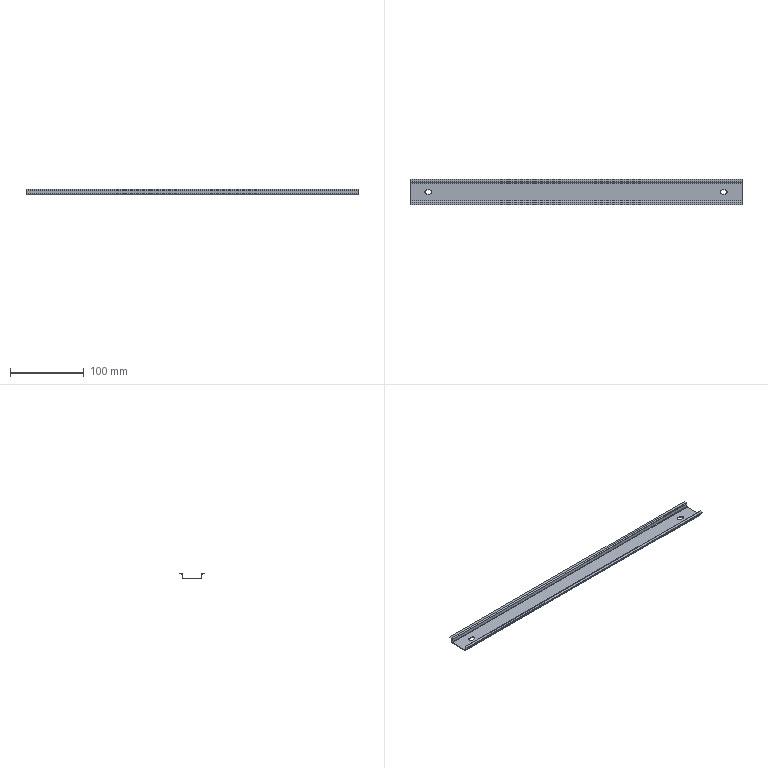Part | SolidWorks | features BaseBody 1 | 1 solid | 48 faces | box 450 x 35 x 7.5 mm | volume 20736 mm3 | plane 34 | cylinder 14 | commonest cylinder face diameters 5.5 x6 1 x4 3 x4
STEP:
#1=CARTESIAN_POINT('',(-202.,-2.75,0.));
#2=VERTEX_POINT('',#1);
#3=CARTESIAN_POINT('',(-198.,-2.75,0.));
#4=VERTEX_POINT('',#3);
#5=CARTESIAN_POINT('',(-202.,-2.75,0.));
#6=DIRECTION('',(1.,0.,0.));
#7=VECTOR('',#6,1000.);
#8=LINE('',#5,#7);
#9=EDGE_CURVE('',#2,#4,#8,.T.);
#10=ORIENTED_EDGE('',*,*,#9,.T.);
#11=CARTESIAN_POINT('',(-198.,-2.75,-1.));
#12=VERTEX_POINT('',#11);
#13=CARTESIAN_POINT('',(-198.,-2.75,-1.));
#14=DIRECTION('',(0.,0.,1.));
#15=VECTOR('',#14,1000.);
#16=LINE('',#13,#15);
#17=EDGE_CURVE('',#12,#4,#16,.T.);
#18=ORIENTED_EDGE('',*,*,#17,.F.);
#19=CARTESIAN_POINT('',(-202.,-2.75,-1.));
#20=VERTEX_POINT('',#19);
#21=CARTESIAN_POINT('',(-202.,-2.75,-1.));
#22=DIRECTION('',(1.,0.,0.));
#23=VECTOR('',#22,1000.);
#24=LINE('',#21,#23);
#25=EDGE_CURVE('',#20,#12,#24,.T.);
#26=ORIENTED_EDGE('',*,*,#25,.F.);
#27=CARTESIAN_POINT('',(-202.,-2.75,-1.));
#28=DIRECTION('',(0.,0.,1.));
#29=VECTOR('',#28,1000.);
#30=LINE('',#27,#29);
#31=EDGE_CURVE('',#20,#2,#30,.T.);
#32=ORIENTED_EDGE('',*,*,#31,.T.);
#33=EDGE_LOOP('',(#10,#18,#26,#32));
#34=FACE_OUTER_BOUND('',#33,.T.);
#35=CARTESIAN_POINT('',(-202.,-2.75,-1.));
#36=DIRECTION('',(0.,-1.,0.));
#37=DIRECTION('',(-1.,0.,0.));
#38=AXIS2_PLACEMENT_3D('',#35,#36,#37);
#39=PLANE('',#38);
#40=ADVANCED_FACE('',(#34),#39,.F.);
#41=CARTESIAN_POINT('',(-195.25,0.,-1.));
#42=VERTEX_POINT('',#41);
#43=CARTESIAN_POINT('',(-195.25,0.,0.));
#44=VERTEX_POINT('',#43);
#45=CARTESIAN_POINT('',(-195.25,0.,-1.));
#46=DIRECTION('',(0.,0.,1.));
#47=VECTOR('',#46,1000.);
#48=LINE('',#45,#47);
#49=EDGE_CURVE('',#42,#44,#48,.T.);
#50=ORIENTED_EDGE('',*,*,#49,.F.);
#51=CARTESIAN_POINT('',(-198.,0.,-1.));
#52=DIRECTION('',(0.,0.,1.));
#53=DIRECTION('',(1.,0.,0.));
#54=AXIS2_PLACEMENT_3D('',#51,#52,#53);
#55=CIRCLE('',#54,2.75);
#56=EDGE_CURVE('',#12,#42,#55,.T.);
#57=ORIENTED_EDGE('',*,*,#56,.F.);
#58=ORIENTED_EDGE('',*,*,#17,.T.);
#59=CARTESIAN_POINT('',(-198.,0.,0.));
#60=DIRECTION('',(0.,0.,1.));
#61=DIRECTION('',(1.,0.,0.));
#62=AXIS2_PLACEMENT_3D('',#59,#60,#61);
#63=CIRCLE('',#62,2.75);
#64=EDGE_CURVE('',#4,#44,#63,.T.);
#65=ORIENTED_EDGE('',*,*,#64,.T.);
#66=EDGE_LOOP('',(#50,#57,#58,#65));
#67=FACE_OUTER_BOUND('',#66,.T.);
#68=CARTESIAN_POINT('',(-198.,0.,-1.));
#69=DIRECTION('',(0.,0.,1.));
#70=DIRECTION('',(1.,0.,0.));
#71=AXIS2_PLACEMENT_3D('',#68,#69,#70);
#72=CYLINDRICAL_SURFACE('',#71,2.75);
#73=ADVANCED_FACE('',(#67),#72,.F.);
#74=CARTESIAN_POINT('',(-198.,2.75,0.));
#75=VERTEX_POINT('',#74);
#76=CARTESIAN_POINT('',(-202.,2.75,0.));
#77=VERTEX_POINT('',#76);
#78=CARTESIAN_POINT('',(-202.,2.75,0.));
#79=DIRECTION('',(-1.,0.,0.));
#80=VECTOR('',#79,1000.);
#81=LINE('',#78,#80);
#82=EDGE_CURVE('',#75,#77,#81,.T.);
#83=ORIENTED_EDGE('',*,*,#82,.T.);
#84=CARTESIAN_POINT('',(-202.,2.75,-1.));
#85=VERTEX_POINT('',#84);
#86=CARTESIAN_POINT('',(-202.,2.75,-1.));
#87=DIRECTION('',(0.,0.,1.));
#88=VECTOR('',#87,1000.);
#89=LINE('',#86,#88);
#90=EDGE_CURVE('',#85,#77,#89,.T.);
#91=ORIENTED_EDGE('',*,*,#90,.F.);
#92=CARTESIAN_POINT('',(-198.,2.75,-1.));
#93=VERTEX_POINT('',#92);
#94=CARTESIAN_POINT('',(-202.,2.75,-1.));
#95=DIRECTION('',(-1.,0.,0.));
#96=VECTOR('',#95,1000.);
#97=LINE('',#94,#96);
#98=EDGE_CURVE('',#93,#85,#97,.T.);
#99=ORIENTED_EDGE('',*,*,#98,.F.);
#100=CARTESIAN_POINT('',(-198.,2.75,-1.));
#101=DIRECTION('',(0.,0.,1.));
#102=VECTOR('',#101,1000.);
#103=LINE('',#100,#102);
#104=EDGE_CURVE('',#93,#75,#103,.T.);
#105=ORIENTED_EDGE('',*,*,#104,.T.);
#106=EDGE_LOOP('',(#83,#91,#99,#105));
#107=FACE_OUTER_BOUND('',#106,.T.);
#108=CARTESIAN_POINT('',(-202.,2.75,-1.));
#109=DIRECTION('',(0.,1.,0.));
#110=DIRECTION('',(1.,0.,0.));
#111=AXIS2_PLACEMENT_3D('',#108,#109,#110);
#112=PLANE('',#111);
#113=ADVANCED_FACE('',(#107),#112,.F.);
#114=CARTESIAN_POINT('',(-202.,0.,0.));
#115=DIRECTION('',(0.,0.,1.));
#116=DIRECTION('',(1.,0.,0.));
#117=AXIS2_PLACEMENT_3D('',#114,#115,#116);
#118=CIRCLE('',#117,2.75);
#119=EDGE_CURVE('',#77,#2,#118,.T.);
#120=ORIENTED_EDGE('',*,*,#119,.T.);
#121=ORIENTED_EDGE('',*,*,#31,.F.);
#122=CARTESIAN_POINT('',(-202.,0.,-1.));
#123=DIRECTION('',(0.,0.,1.));
#124=DIRECTION('',(1.,0.,0.));
#125=AXIS2_PLACEMENT_3D('',#122,#123,#124);
#126=CIRCLE('',#125,2.75);
#127=EDGE_CURVE('',#85,#20,#126,.T.);
#128=ORIENTED_EDGE('',*,*,#127,.F.);
#129=ORIENTED_EDGE('',*,*,#90,.T.);
#130=EDGE_LOOP('',(#120,#121,#128,#129));
#131=FACE_OUTER_BOUND('',#130,.T.);
#132=CARTESIAN_POINT('',(-202.,0.,-1.));
#133=DIRECTION('',(0.,0.,1.));
#134=DIRECTION('',(1.,0.,0.));
#135=AXIS2_PLACEMENT_3D('',#132,#133,#134);
#136=CYLINDRICAL_SURFACE('',#135,2.75);
#137=ADVANCED_FACE('',(#131),#136,.F.);
#138=CARTESIAN_POINT('',(202.,2.75,0.));
#139=VERTEX_POINT('',#138);
#140=CARTESIAN_POINT('',(198.,2.75,0.));
#141=VERTEX_POINT('',#140);
#142=CARTESIAN_POINT('',(202.,2.75,0.));
#143=DIRECTION('',(-1.,0.,0.));
#144=VECTOR('',#143,1000.);
#145=LINE('',#142,#144);
#146=EDGE_CURVE('',#139,#141,#145,.T.);
#147=ORIENTED_EDGE('',*,*,#146,.T.);
#148=CARTESIAN_POINT('',(198.,2.75,-1.));
#149=VERTEX_POINT('',#148);
#150=CARTESIAN_POINT('',(198.,2.75,-1.));
#151=DIRECTION('',(0.,0.,1.));
#152=VECTOR('',#151,1000.);
#153=LINE('',#150,#152);
#154=EDGE_CURVE('',#149,#141,#153,.T.);
#155=ORIENTED_EDGE('',*,*,#154,.F.);
#156=CARTESIAN_POINT('',(202.,2.75,-1.));
#157=VERTEX_POINT('',#156);
#158=CARTESIAN_POINT('',(202.,2.75,-1.));
#159=DIRECTION('',(-1.,0.,0.));
#160=VECTOR('',#159,1000.);
#161=LINE('',#158,#160);
#162=EDGE_CURVE('',#157,#149,#161,.T.);
#163=ORIENTED_EDGE('',*,*,#162,.F.);
#164=CARTESIAN_POINT('',(202.,2.75,-1.));
#165=DIRECTION('',(0.,0.,1.));
#166=VECTOR('',#165,1000.);
#167=LINE('',#164,#166);
#168=EDGE_CURVE('',#157,#139,#167,.T.);
#169=ORIENTED_EDGE('',*,*,#168,.T.);
#170=EDGE_LOOP('',(#147,#155,#163,#169));
#171=FACE_OUTER_BOUND('',#170,.T.);
#172=CARTESIAN_POINT('',(202.,2.75,-1.));
#173=DIRECTION('',(0.,1.,0.));
#174=DIRECTION('',(1.,0.,0.));
#175=AXIS2_PLACEMENT_3D('',#172,#173,#174);
#176=PLANE('',#175);
#177=ADVANCED_FACE('',(#171),#176,.F.);
#178=CARTESIAN_POINT('',(198.,-2.75,0.));
#179=VERTEX_POINT('',#178);
#180=CARTESIAN_POINT('',(198.,0.,0.));
#181=DIRECTION('',(0.,0.,1.));
#182=DIRECTION('',(-1.,0.,0.));
#183=AXIS2_PLACEMENT_3D('',#180,#181,#182);
#184=CIRCLE('',#183,2.75);
#185=EDGE_CURVE('',#141,#179,#184,.T.);
#186=ORIENTED_EDGE('',*,*,#185,.T.);
#187=CARTESIAN_POINT('',(198.,-2.75,-1.));
#188=VERTEX_POINT('',#187);
#189=CARTESIAN_POINT('',(198.,-2.75,-1.));
#190=DIRECTION('',(0.,0.,1.));
#191=VECTOR('',#190,1000.);
#192=LINE('',#189,#191);
#193=EDGE_CURVE('',#188,#179,#192,.T.);
#194=ORIENTED_EDGE('',*,*,#193,.F.);
#195=CARTESIAN_POINT('',(198.,0.,-1.));
#196=DIRECTION('',(0.,0.,1.));
#197=DIRECTION('',(-1.,0.,0.));
#198=AXIS2_PLACEMENT_3D('',#195,#196,#197);
#199=CIRCLE('',#198,2.75);
#200=EDGE_CURVE('',#149,#188,#199,.T.);
#201=ORIENTED_EDGE('',*,*,#200,.F.);
#202=ORIENTED_EDGE('',*,*,#154,.T.);
#203=EDGE_LOOP('',(#186,#194,#201,#202));
#204=FACE_OUTER_BOUND('',#203,.T.);
#205=CARTESIAN_POINT('',(198.,0.,-1.));
#206=DIRECTION('',(0.,0.,1.));
#207=DIRECTION('',(1.,0.,0.));
#208=AXIS2_PLACEMENT_3D('',#205,#206,#207);
#209=CYLINDRICAL_SURFACE('',#208,2.75);
#210=ADVANCED_FACE('',(#204),#209,.F.);
#211=CARTESIAN_POINT('',(202.,-2.75,0.));
#212=VERTEX_POINT('',#211);
#213=CARTESIAN_POINT('',(202.,-2.75,0.));
#214=DIRECTION('',(1.,0.,0.));
#215=VECTOR('',#214,1000.);
#216=LINE('',#213,#215);
#217=EDGE_CURVE('',#179,#212,#216,.T.);
#218=ORIENTED_EDGE('',*,*,#217,.T.);
#219=CARTESIAN_POINT('',(202.,-2.75,-1.));
#220=VERTEX_POINT('',#219);
#221=CARTESIAN_POINT('',(202.,-2.75,-1.));
#222=DIRECTION('',(0.,0.,1.));
#223=VECTOR('',#222,1000.);
#224=LINE('',#221,#223);
#225=EDGE_CURVE('',#220,#212,#224,.T.);
#226=ORIENTED_EDGE('',*,*,#225,.F.);
#227=CARTESIAN_POINT('',(202.,-2.75,-1.));
#228=DIRECTION('',(1.,0.,0.));
#229=VECTOR('',#228,1000.);
#230=LINE('',#227,#229);
#231=EDGE_CURVE('',#188,#220,#230,.T.);
#232=ORIENTED_EDGE('',*,*,#231,.F.);
#233=ORIENTED_EDGE('',*,*,#193,.T.);
#234=EDGE_LOOP('',(#218,#226,#232,#233));
#235=FACE_OUTER_BOUND('',#234,.T.);
#236=CARTESIAN_POINT('',(202.,-2.75,-1.));
#237=DIRECTION('',(0.,-1.,0.));
#238=DIRECTION('',(0.,0.,-1.));
#239=AXIS2_PLACEMENT_3D('',#236,#237,#238);
#240=PLANE('',#239);
#241=ADVANCED_FACE('',(#235),#240,.F.);
#242=CARTESIAN_POINT('',(204.75,0.,-1.));
#243=VERTEX_POINT('',#242);
#244=CARTESIAN_POINT('',(204.75,0.,0.));
#245=VERTEX_POINT('',#244);
#246=CARTESIAN_POINT('',(204.75,0.,-1.));
#247=DIRECTION('',(0.,0.,1.));
#248=VECTOR('',#247,1000.);
#249=LINE('',#246,#248);
#250=EDGE_CURVE('',#243,#245,#249,.T.);
#251=ORIENTED_EDGE('',*,*,#250,.F.);
#252=CARTESIAN_POINT('',(202.,0.,-1.));
#253=DIRECTION('',(0.,0.,1.));
#254=DIRECTION('',(-1.,0.,0.));
#255=AXIS2_PLACEMENT_3D('',#252,#253,#254);
#256=CIRCLE('',#255,2.75);
#257=EDGE_CURVE('',#220,#243,#256,.T.);
#258=ORIENTED_EDGE('',*,*,#257,.F.);
#259=ORIENTED_EDGE('',*,*,#225,.T.);
#260=CARTESIAN_POINT('',(202.,0.,0.));
#261=DIRECTION('',(0.,0.,1.));
#262=DIRECTION('',(-1.,0.,0.));
#263=AXIS2_PLACEMENT_3D('',#260,#261,#262);
#264=CIRCLE('',#263,2.75);
#265=EDGE_CURVE('',#212,#245,#264,.T.);
#266=ORIENTED_EDGE('',*,*,#265,.T.);
#267=EDGE_LOOP('',(#251,#258,#259,#266));
#268=FACE_OUTER_BOUND('',#267,.T.);
#269=CARTESIAN_POINT('',(202.,0.,-1.));
#270=DIRECTION('',(0.,0.,1.));
#271=DIRECTION('',(1.,0.,0.));
#272=AXIS2_PLACEMENT_3D('',#269,#270,#271);
#273=CYLINDRICAL_SURFACE('',#272,2.75);
#274=ADVANCED_FACE('',(#268),#273,.F.);
#275=CARTESIAN_POINT('',(-225.,-17.5,5.5));
#276=VERTEX_POINT('',#275);
#277=CARTESIAN_POINT('',(225.,-17.5,5.5));
#278=VERTEX_POINT('',#277);
#279=CARTESIAN_POINT('',(225.,-17.5,5.5));
#280=DIRECTION('',(1.,0.,0.));
#281=VECTOR('',#280,1000.);
#282=LINE('',#279,#281);
#283=EDGE_CURVE('',#276,#278,#282,.T.);
#284=ORIENTED_EDGE('',*,*,#283,.T.);
#285=CARTESIAN_POINT('',(225.,-17.5,6.5));
#286=VERTEX_POINT('',#285);
#287=CARTESIAN_POINT('',(225.,-17.5,6.5));
#288=DIRECTION('',(0.,0.,-1.));
#289=VECTOR('',#288,1000.);
#290=LINE('',#287,#289);
#291=EDGE_CURVE('',#286,#278,#290,.T.);
#292=ORIENTED_EDGE('',*,*,#291,.F.);
#293=CARTESIAN_POINT('',(-225.,-17.5,6.5));
#294=VERTEX_POINT('',#293);
#295=CARTESIAN_POINT('',(0.,-17.5,6.5));
#296=DIRECTION('',(1.,0.,0.));
#297=VECTOR('',#296,1000.);
#298=LINE('',#295,#297);
#299=EDGE_CURVE('',#294,#286,#298,.T.);
#300=ORIENTED_EDGE('',*,*,#299,.F.);
#301=CARTESIAN_POINT('',(-225.,-17.5,6.5));
#302=DIRECTION('',(0.,0.,-1.));
#303=VECTOR('',#302,1000.);
#304=LINE('',#301,#303);
#305=EDGE_CURVE('',#294,#276,#304,.T.);
#306=ORIENTED_EDGE('',*,*,#305,.T.);
#307=EDGE_LOOP('',(#284,#292,#300,#306));
#308=FACE_OUTER_BOUND('',#307,.T.);
#309=CARTESIAN_POINT('',(225.,-17.5,6.5));
#310=DIRECTION('',(0.,1.,0.));
#311=DIRECTION('',(1.,0.,0.));
#312=AXIS2_PLACEMENT_3D('',#309,#310,#311);
#313=PLANE('',#312);
#314=ADVANCED_FACE('',(#308),#313,.F.);
#315=CARTESIAN_POINT('',(-225.,-14.,5.5));
#316=VERTEX_POINT('',#315);
#317=CARTESIAN_POINT('',(-225.,-17.5,5.5));
#318=DIRECTION('',(0.,-1.,0.));
#319=VECTOR('',#318,1000.);
#320=LINE('',#317,#319);
#321=EDGE_CURVE('',#316,#276,#320,.T.);
#322=ORIENTED_EDGE('',*,*,#321,.F.);
#323=CARTESIAN_POINT('',(225.,-14.,5.5));
#324=VERTEX_POINT('',#323);
#325=CARTESIAN_POINT('',(225.,-14.,5.5));
#326=DIRECTION('',(-1.,0.,0.));
#327=VECTOR('',#326,1000.);
#328=LINE('',#325,#327);
#329=EDGE_CURVE('',#324,#316,#328,.T.);
#330=ORIENTED_EDGE('',*,*,#329,.F.);
#331=CARTESIAN_POINT('',(225.,-13.5,5.5));
#332=DIRECTION('',(0.,1.,0.));
#333=VECTOR('',#332,1000.);
#334=LINE('',#331,#333);
#335=EDGE_CURVE('',#278,#324,#334,.T.);
#336=ORIENTED_EDGE('',*,*,#335,.F.);
#337=ORIENTED_EDGE('',*,*,#283,.F.);
#338=EDGE_LOOP('',(#322,#330,#336,#337));
#339=FACE_OUTER_BOUND('',#338,.T.);
#340=CARTESIAN_POINT('',(0.,0.,5.5));
#341=DIRECTION('',(0.,0.,-1.));
#342=DIRECTION('',(0.,-1.,0.));
#343=AXIS2_PLACEMENT_3D('',#340,#341,#342);
#344=PLANE('',#343);
#345=ADVANCED_FACE('',(#339),#344,.T.);
#346=CARTESIAN_POINT('',(-225.,-14.,6.5));
#347=VERTEX_POINT('',#346);
#348=CARTESIAN_POINT('',(225.,-14.,6.5));
#349=VERTEX_POINT('',#348);
#350=CARTESIAN_POINT('',(225.,-14.,6.5));
#351=DIRECTION('',(1.,0.,0.));
#352=VECTOR('',#351,1000.);
#353=LINE('',#350,#352);
#354=EDGE_CURVE('',#347,#349,#353,.T.);
#355=ORIENTED_EDGE('',*,*,#354,.F.);
#356=CARTESIAN_POINT('',(-225.,0.,6.5));
#357=DIRECTION('',(0.,-1.,0.));
#358=VECTOR('',#357,1000.);
#359=LINE('',#356,#358);
#360=EDGE_CURVE('',#347,#294,#359,.T.);
#361=ORIENTED_EDGE('',*,*,#360,.T.);
#362=ORIENTED_EDGE('',*,*,#299,.T.);
#363=CARTESIAN_POINT('',(225.,0.,6.5));
#364=DIRECTION('',(0.,1.,0.));
#365=VECTOR('',#364,1000.);
#366=LINE('',#363,#365);
#367=EDGE_CURVE('',#286,#349,#366,.T.);
#368=ORIENTED_EDGE('',*,*,#367,.T.);
#369=EDGE_LOOP('',(#355,#361,#362,#368));
#370=FACE_OUTER_BOUND('',#369,.T.);
#371=CARTESIAN_POINT('',(0.,0.,6.5));
#372=DIRECTION('',(0.,0.,-1.));
#373=DIRECTION('',(0.,-1.,0.));
#374=AXIS2_PLACEMENT_3D('',#371,#372,#373);
#375=PLANE('',#374);
#376=ADVANCED_FACE('',(#370),#375,.F.);
#377=CARTESIAN_POINT('',(-225.,-14.,5.5));
#378=DIRECTION('',(0.,0.,1.));
#379=VECTOR('',#378,1000.);
#380=LINE('',#377,#379);
#381=EDGE_CURVE('',#316,#347,#380,.T.);
#382=ORIENTED_EDGE('',*,*,#381,.F.);
#383=ORIENTED_EDGE('',*,*,#321,.T.);
#384=ORIENTED_EDGE('',*,*,#305,.F.);
#385=ORIENTED_EDGE('',*,*,#360,.F.);
#386=EDGE_LOOP('',(#382,#383,#384,#385));
#387=FACE_OUTER_BOUND('',#386,.T.);
#388=CARTESIAN_POINT('',(-225.,-17.5,6.5));
#389=DIRECTION('',(1.,0.,0.));
#390=DIRECTION('',(0.,0.,1.));
#391=AXIS2_PLACEMENT_3D('',#388,#389,#390);
#392=PLANE('',#391);
#393=ADVANCED_FACE('',(#387),#392,.F.);
#394=CARTESIAN_POINT('',(225.,-14.,6.5));
#395=DIRECTION('',(0.,0.,1.));
#396=VECTOR('',#395,1000.);
#397=LINE('',#394,#396);
#398=EDGE_CURVE('',#324,#349,#397,.T.);
#399=ORIENTED_EDGE('',*,*,#398,.T.);
#400=ORIENTED_EDGE('',*,*,#367,.F.);
#401=ORIENTED_EDGE('',*,*,#291,.T.);
#402=ORIENTED_EDGE('',*,*,#335,.T.);
#403=EDGE_LOOP('',(#399,#400,#401,#402));
#404=FACE_OUTER_BOUND('',#403,.T.);
#405=CARTESIAN_POINT('',(225.,-13.5,6.5));
#406=DIRECTION('',(-1.,0.,0.));
#407=DIRECTION('',(0.,0.,1.));
#408=AXIS2_PLACEMENT_3D('',#405,#406,#407);
#409=PLANE('',#408);
#410=ADVANCED_FACE('',(#404),#409,.F.);
#411=CARTESIAN_POINT('',(-225.,-13.5,5.));
#412=VERTEX_POINT('',#411);
#413=CARTESIAN_POINT('',(225.,-13.5,5.));
#414=VERTEX_POINT('',#413);
#415=CARTESIAN_POINT('',(-225.,-13.5,5.));
#416=DIRECTION('',(1.,0.,0.));
#417=VECTOR('',#416,1000.);
#418=LINE('',#415,#417);
#419=EDGE_CURVE('',#412,#414,#418,.T.);
#420=ORIENTED_EDGE('',*,*,#419,.T.);
#421=CARTESIAN_POINT('',(225.,-14.,5.));
#422=DIRECTION('',(1.,0.,0.));
#423=DIRECTION('',(0.,0.,1.));
#424=AXIS2_PLACEMENT_3D('',#421,#422,#423);
#425=CIRCLE('',#424,0.5);
#426=EDGE_CURVE('',#414,#324,#425,.T.);
#427=ORIENTED_EDGE('',*,*,#426,.T.);
#428=ORIENTED_EDGE('',*,*,#329,.T.);
#429=CARTESIAN_POINT('',(-225.,-14.,5.));
#430=DIRECTION('',(-1.,0.,0.));
#431=DIRECTION('',(0.,0.,1.));
#432=AXIS2_PLACEMENT_3D('',#429,#430,#431);
#433=CIRCLE('',#432,0.5);
#434=EDGE_CURVE('',#316,#412,#433,.T.);
#435=ORIENTED_EDGE('',*,*,#434,.T.);
#436=EDGE_LOOP('',(#420,#427,#428,#435));
#437=FACE_OUTER_BOUND('',#436,.T.);
#438=CARTESIAN_POINT('',(-225.,-14.,5.));
#439=DIRECTION('',(-1.,0.,0.));
#440=DIRECTION('',(0.,0.,1.));
#441=AXIS2_PLACEMENT_3D('',#438,#439,#440);
#442=CYLINDRICAL_SURFACE('',#441,0.5);
#443=ADVANCED_FACE('',(#437),#442,.F.);
#444=CARTESIAN_POINT('',(-225.,-12.5,5.));
#445=VERTEX_POINT('',#444);
#446=CARTESIAN_POINT('',(225.,-12.5,5.));
#447=VERTEX_POINT('',#446);
#448=CARTESIAN_POINT('',(-225.,-12.5,5.));
#449=DIRECTION('',(1.,0.,0.));
#450=VECTOR('',#449,1000.);
#451=LINE('',#448,#450);
#452=EDGE_CURVE('',#445,#447,#451,.T.);
#453=ORIENTED_EDGE('',*,*,#452,.F.);
#454=CARTESIAN_POINT('',(-225.,-14.,5.));
#455=DIRECTION('',(-1.,0.,0.));
#456=DIRECTION('',(0.,0.,1.));
#457=AXIS2_PLACEMENT_3D('',#454,#455,#456);
#458=CIRCLE('',#457,1.5);
#459=EDGE_CURVE('',#347,#445,#458,.T.);
#460=ORIENTED_EDGE('',*,*,#459,.F.);
#461=ORIENTED_EDGE('',*,*,#354,.T.);
#462=CARTESIAN_POINT('',(225.,-14.,5.));
#463=DIRECTION('',(1.,0.,0.));
#464=DIRECTION('',(0.,0.,1.));
#465=AXIS2_PLACEMENT_3D('',#462,#463,#464);
#466=CIRCLE('',#465,1.5);
#467=EDGE_CURVE('',#447,#349,#466,.T.);
#468=ORIENTED_EDGE('',*,*,#467,.F.);
#469=EDGE_LOOP('',(#453,#460,#461,#468));
#470=FACE_OUTER_BOUND('',#469,.T.);
#471=CARTESIAN_POINT('',(-225.,-14.,5.));
#472=DIRECTION('',(-1.,0.,0.));
#473=DIRECTION('',(0.,0.,1.));
#474=AXIS2_PLACEMENT_3D('',#471,#472,#473);
#475=CYLINDRICAL_SURFACE('',#474,1.5);
#476=ADVANCED_FACE('',(#470),#475,.T.);
#477=ORIENTED_EDGE('',*,*,#434,.F.);
#478=ORIENTED_EDGE('',*,*,#381,.T.);
#479=ORIENTED_EDGE('',*,*,#459,.T.);
#480=CARTESIAN_POINT('',(-225.,-13.5,5.));
#481=DIRECTION('',(0.,1.,0.));
#482=VECTOR('',#481,1000.);
#483=LINE('',#480,#482);
#484=EDGE_CURVE('',#412,#445,#483,.T.);
#485=ORIENTED_EDGE('',*,*,#484,.F.);
#486=EDGE_LOOP('',(#477,#478,#479,#485));
#487=FACE_OUTER_BOUND('',#486,.T.);
#488=CARTESIAN_POINT('',(-225.,-14.,5.));
#489=DIRECTION('',(1.,0.,0.));
#490=DIRECTION('',(0.,1.,0.));
#491=AXIS2_PLACEMENT_3D('',#488,#489,#490);
#492=PLANE('',#491);
#493=ADVANCED_FACE('',(#487),#492,.F.);
#494=ORIENTED_EDGE('',*,*,#398,.F.);
#495=ORIENTED_EDGE('',*,*,#426,.F.);
#496=CARTESIAN_POINT('',(225.,-13.5,5.));
#497=DIRECTION('',(0.,1.,0.));
#498=VECTOR('',#497,1000.);
#499=LINE('',#496,#498);
#500=EDGE_CURVE('',#414,#447,#499,.T.);
#501=ORIENTED_EDGE('',*,*,#500,.T.);
#502=ORIENTED_EDGE('',*,*,#467,.T.);
#503=EDGE_LOOP('',(#494,#495,#501,#502));
#504=FACE_OUTER_BOUND('',#503,.T.);
#505=CARTESIAN_POINT('',(225.,-14.,5.));
#506=DIRECTION('',(1.,0.,0.));
#507=DIRECTION('',(0.,1.,0.));
#508=AXIS2_PLACEMENT_3D('',#505,#506,#507);
#509=PLANE('',#508);
#510=ADVANCED_FACE('',(#504),#509,.T.);
#511=CARTESIAN_POINT('',(225.,17.5,5.5));
#512=VERTEX_POINT('',#511);
#513=CARTESIAN_POINT('',(-225.,17.5,5.5));
#514=VERTEX_POINT('',#513);
#515=CARTESIAN_POINT('',(-225.,17.5,5.5));
#516=DIRECTION('',(-1.,0.,0.));
#517=VECTOR('',#516,1000.);
#518=LINE('',#515,#517);
#519=EDGE_CURVE('',#512,#514,#518,.T.);
#520=ORIENTED_EDGE('',*,*,#519,.T.);
#521=CARTESIAN_POINT('',(-225.,17.5,6.5));
#522=VERTEX_POINT('',#521);
#523=CARTESIAN_POINT('',(-225.,17.5,6.5));
#524=DIRECTION('',(0.,0.,-1.));
#525=VECTOR('',#524,1000.);
#526=LINE('',#523,#525);
#527=EDGE_CURVE('',#522,#514,#526,.T.);
#528=ORIENTED_EDGE('',*,*,#527,.F.);
#529=CARTESIAN_POINT('',(225.,17.5,6.5));
#530=VERTEX_POINT('',#529);
#531=CARTESIAN_POINT('',(0.,17.5,6.5));
#532=DIRECTION('',(-1.,0.,0.));
#533=VECTOR('',#532,1000.);
#534=LINE('',#531,#533);
#535=EDGE_CURVE('',#530,#522,#534,.T.);
#536=ORIENTED_EDGE('',*,*,#535,.F.);
#537=CARTESIAN_POINT('',(225.,17.5,6.5));
#538=DIRECTION('',(0.,0.,-1.));
#539=VECTOR('',#538,1000.);
#540=LINE('',#537,#539);
#541=EDGE_CURVE('',#530,#512,#540,.T.);
#542=ORIENTED_EDGE('',*,*,#541,.T.);
#543=EDGE_LOOP('',(#520,#528,#536,#542));
#544=FACE_OUTER_BOUND('',#543,.T.);
#545=CARTESIAN_POINT('',(-225.,17.5,6.5));
#546=DIRECTION('',(0.,-1.,0.));
#547=DIRECTION('',(0.,0.,-1.));
#548=AXIS2_PLACEMENT_3D('',#545,#546,#547);
#549=PLANE('',#548);
#550=ADVANCED_FACE('',(#544),#549,.F.);
#551=CARTESIAN_POINT('',(225.,14.,5.5));
#552=VERTEX_POINT('',#551);
#553=CARTESIAN_POINT('',(225.,17.5,5.5));
#554=DIRECTION('',(0.,1.,0.));
#555=VECTOR('',#554,1000.);
#556=LINE('',#553,#555);
#557=EDGE_CURVE('',#552,#512,#556,.T.);
#558=ORIENTED_EDGE('',*,*,#557,.F.);
#559=CARTESIAN_POINT('',(-225.,14.,5.5));
#560=VERTEX_POINT('',#559);
#561=CARTESIAN_POINT('',(-225.,14.,5.5));
#562=DIRECTION('',(1.,0.,0.));
#563=VECTOR('',#562,1000.);
#564=LINE('',#561,#563);
#565=EDGE_CURVE('',#560,#552,#564,.T.);
#566=ORIENTED_EDGE('',*,*,#565,.F.);
#567=CARTESIAN_POINT('',(-225.,13.5,5.5));
#568=DIRECTION('',(0.,-1.,0.));
#569=VECTOR('',#568,1000.);
#570=LINE('',#567,#569);
#571=EDGE_CURVE('',#514,#560,#570,.T.);
#572=ORIENTED_EDGE('',*,*,#571,.F.);
#573=ORIENTED_EDGE('',*,*,#519,.F.);
#574=EDGE_LOOP('',(#558,#566,#572,#573));
#575=FACE_OUTER_BOUND('',#574,.T.);
#576=CARTESIAN_POINT('',(0.,0.,5.5));
#577=DIRECTION('',(0.,0.,-1.));
#578=DIRECTION('',(0.,-1.,0.));
#579=AXIS2_PLACEMENT_3D('',#576,#577,#578);
#580=PLANE('',#579);
#581=ADVANCED_FACE('',(#575),#580,.T.);
#582=CARTESIAN_POINT('',(225.,14.,6.5));
#583=VERTEX_POINT('',#582);
#584=CARTESIAN_POINT('',(-225.,14.,6.5));
#585=VERTEX_POINT('',#584);
#586=CARTESIAN_POINT('',(-225.,14.,6.5));
#587=DIRECTION('',(-1.,0.,0.));
#588=VECTOR('',#587,1000.);
#589=LINE('',#586,#588);
#590=EDGE_CURVE('',#583,#585,#589,.T.);
#591=ORIENTED_EDGE('',*,*,#590,.F.);
#592=CARTESIAN_POINT('',(225.,0.,6.5));
#593=DIRECTION('',(0.,1.,0.));
#594=VECTOR('',#593,1000.);
#595=LINE('',#592,#594);
#596=EDGE_CURVE('',#583,#530,#595,.T.);
#597=ORIENTED_EDGE('',*,*,#596,.T.);
#598=ORIENTED_EDGE('',*,*,#535,.T.);
#599=CARTESIAN_POINT('',(-225.,0.,6.5));
#600=DIRECTION('',(0.,-1.,0.));
#601=VECTOR('',#600,1000.);
#602=LINE('',#599,#601);
#603=EDGE_CURVE('',#522,#585,#602,.T.);
#604=ORIENTED_EDGE('',*,*,#603,.T.);
#605=EDGE_LOOP('',(#591,#597,#598,#604));
#606=FACE_OUTER_BOUND('',#605,.T.);
#607=CARTESIAN_POINT('',(0.,0.,6.5));
#608=DIRECTION('',(0.,0.,-1.));
#609=DIRECTION('',(0.,-1.,0.));
#610=AXIS2_PLACEMENT_3D('',#607,#608,#609);
#611=PLANE('',#610);
#612=ADVANCED_FACE('',(#606),#611,.F.);
#613=CARTESIAN_POINT('',(225.,14.,5.5));
#614=DIRECTION('',(0.,0.,1.));
#615=VECTOR('',#614,1000.);
#616=LINE('',#613,#615);
#617=EDGE_CURVE('',#552,#583,#616,.T.);
#618=ORIENTED_EDGE('',*,*,#617,.F.);
#619=ORIENTED_EDGE('',*,*,#557,.T.);
#620=ORIENTED_EDGE('',*,*,#541,.F.);
#621=ORIENTED_EDGE('',*,*,#596,.F.);
#622=EDGE_LOOP('',(#618,#619,#620,#621));
#623=FACE_OUTER_BOUND('',#622,.T.);
#624=CARTESIAN_POINT('',(225.,17.5,6.5));
#625=DIRECTION('',(-1.,0.,0.));
#626=DIRECTION('',(0.,0.,1.));
#627=AXIS2_PLACEMENT_3D('',#624,#625,#626);
#628=PLANE('',#627);
#629=ADVANCED_FACE('',(#623),#628,.F.);
#630=CARTESIAN_POINT('',(-225.,14.,6.5));
#631=DIRECTION('',(0.,0.,1.));
#632=VECTOR('',#631,1000.);
#633=LINE('',#630,#632);
#634=EDGE_CURVE('',#560,#585,#633,.T.);
#635=ORIENTED_EDGE('',*,*,#634,.T.);
#636=ORIENTED_EDGE('',*,*,#603,.F.);
#637=ORIENTED_EDGE('',*,*,#527,.T.);
#638=ORIENTED_EDGE('',*,*,#571,.T.);
#639=EDGE_LOOP('',(#635,#636,#637,#638));
#640=FACE_OUTER_BOUND('',#639,.T.);
#641=CARTESIAN_POINT('',(-225.,13.5,6.5));
#642=DIRECTION('',(1.,0.,0.));
#643=DIRECTION('',(0.,1.,0.));
#644=AXIS2_PLACEMENT_3D('',#641,#642,#643);
#645=PLANE('',#644);
#646=ADVANCED_FACE('',(#640),#645,.F.);
#647=CARTESIAN_POINT('',(225.,13.5,5.));
#648=VERTEX_POINT('',#647);
#649=CARTESIAN_POINT('',(-225.,13.5,5.));
#650=VERTEX_POINT('',#649);
#651=CARTESIAN_POINT('',(225.,13.5,5.));
#652=DIRECTION('',(-1.,0.,0.));
#653=VECTOR('',#652,1000.);
#654=LINE('',#651,#653);
#655=EDGE_CURVE('',#648,#650,#654,.T.);
#656=ORIENTED_EDGE('',*,*,#655,.T.);
#657=CARTESIAN_POINT('',(-225.,14.,5.));
#658=DIRECTION('',(-1.,0.,0.));
#659=DIRECTION('',(0.,0.,-1.));
#660=AXIS2_PLACEMENT_3D('',#657,#658,#659);
#661=CIRCLE('',#660,0.5);
#662=EDGE_CURVE('',#650,#560,#661,.T.);
#663=ORIENTED_EDGE('',*,*,#662,.T.);
#664=ORIENTED_EDGE('',*,*,#565,.T.);
#665=CARTESIAN_POINT('',(225.,14.,5.));
#666=DIRECTION('',(1.,0.,0.));
#667=DIRECTION('',(0.,0.,-1.));
#668=AXIS2_PLACEMENT_3D('',#665,#666,#667);
#669=CIRCLE('',#668,0.5);
#670=EDGE_CURVE('',#552,#648,#669,.T.);
#671=ORIENTED_EDGE('',*,*,#670,.T.);
#672=EDGE_LOOP('',(#656,#663,#664,#671));
#673=FACE_OUTER_BOUND('',#672,.T.);
#674=CARTESIAN_POINT('',(225.,14.,5.));
#675=DIRECTION('',(1.,0.,0.));
#676=DIRECTION('',(0.,0.,1.));
#677=AXIS2_PLACEMENT_3D('',#674,#675,#676);
#678=CYLINDRICAL_SURFACE('',#677,0.5);
#679=ADVANCED_FACE('',(#673),#678,.F.);
#680=CARTESIAN_POINT('',(225.,12.5,5.));
#681=VERTEX_POINT('',#680);
#682=CARTESIAN_POINT('',(-225.,12.5,5.));
#683=VERTEX_POINT('',#682);
#684=CARTESIAN_POINT('',(225.,12.5,5.));
#685=DIRECTION('',(-1.,0.,0.));
#686=VECTOR('',#685,1000.);
#687=LINE('',#684,#686);
#688=EDGE_CURVE('',#681,#683,#687,.T.);
#689=ORIENTED_EDGE('',*,*,#688,.F.);
#690=CARTESIAN_POINT('',(225.,14.,5.));
#691=DIRECTION('',(1.,0.,0.));
#692=DIRECTION('',(0.,0.,-1.));
#693=AXIS2_PLACEMENT_3D('',#690,#691,#692);
#694=CIRCLE('',#693,1.5);
#695=EDGE_CURVE('',#583,#681,#694,.T.);
#696=ORIENTED_EDGE('',*,*,#695,.F.);
#697=ORIENTED_EDGE('',*,*,#590,.T.);
#698=CARTESIAN_POINT('',(-225.,14.,5.));
#699=DIRECTION('',(-1.,0.,0.));
#700=DIRECTION('',(0.,0.,-1.));
#701=AXIS2_PLACEMENT_3D('',#698,#699,#700);
#702=CIRCLE('',#701,1.5);
#703=EDGE_CURVE('',#683,#585,#702,.T.);
#704=ORIENTED_EDGE('',*,*,#703,.F.);
#705=EDGE_LOOP('',(#689,#696,#697,#704));
#706=FACE_OUTER_BOUND('',#705,.T.);
#707=CARTESIAN_POINT('',(225.,14.,5.));
#708=DIRECTION('',(1.,0.,0.));
#709=DIRECTION('',(0.,0.,1.));
#710=AXIS2_PLACEMENT_3D('',#707,#708,#709);
#711=CYLINDRICAL_SURFACE('',#710,1.5);
#712=ADVANCED_FACE('',(#706),#711,.T.);
#713=ORIENTED_EDGE('',*,*,#670,.F.);
#714=ORIENTED_EDGE('',*,*,#617,.T.);
#715=ORIENTED_EDGE('',*,*,#695,.T.);
#716=CARTESIAN_POINT('',(225.,13.5,5.));
#717=DIRECTION('',(0.,-1.,0.));
#718=VECTOR('',#717,1000.);
#719=LINE('',#716,#718);
#720=EDGE_CURVE('',#648,#681,#719,.T.);
#721=ORIENTED_EDGE('',*,*,#720,.F.);
#722=EDGE_LOOP('',(#713,#714,#715,#721));
#723=FACE_OUTER_BOUND('',#722,.T.);
#724=CARTESIAN_POINT('',(225.,14.,5.));
#725=DIRECTION('',(-1.,0.,0.));
#726=DIRECTION('',(0.,0.,1.));
#727=AXIS2_PLACEMENT_3D('',#724,#725,#726);
#728=PLANE('',#727);
#729=ADVANCED_FACE('',(#723),#728,.F.);
#730=ORIENTED_EDGE('',*,*,#634,.F.);
#731=ORIENTED_EDGE('',*,*,#662,.F.);
#732=CARTESIAN_POINT('',(-225.,13.5,5.));
#733=DIRECTION('',(0.,-1.,0.));
#734=VECTOR('',#733,1000.);
#735=LINE('',#732,#734);
#736=EDGE_CURVE('',#650,#683,#735,.T.);
#737=ORIENTED_EDGE('',*,*,#736,.T.);
#738=ORIENTED_EDGE('',*,*,#703,.T.);
#739=EDGE_LOOP('',(#730,#731,#737,#738));
#740=FACE_OUTER_BOUND('',#739,.T.);
#741=CARTESIAN_POINT('',(-225.,14.,5.));
#742=DIRECTION('',(-1.,0.,0.));
#743=DIRECTION('',(0.,0.,1.));
#744=AXIS2_PLACEMENT_3D('',#741,#742,#743);
#745=PLANE('',#744);
#746=ADVANCED_FACE('',(#740),#745,.T.);
#747=CARTESIAN_POINT('',(225.,-12.,0.));
#748=VERTEX_POINT('',#747);
#749=CARTESIAN_POINT('',(-225.,-12.,0.));
#750=VERTEX_POINT('',#749);
#751=CARTESIAN_POINT('',(225.,-12.,0.));
#752=DIRECTION('',(-1.,0.,0.));
#753=VECTOR('',#752,1000.);
#754=LINE('',#751,#753);
#755=EDGE_CURVE('',#748,#750,#754,.T.);
#756=ORIENTED_EDGE('',*,*,#755,.T.);
#757=CARTESIAN_POINT('',(-225.,-12.5,0.5));
#758=VERTEX_POINT('',#757);
#759=CARTESIAN_POINT('',(-225.,-12.,0.5));
#760=DIRECTION('',(-1.,0.,0.));
#761=DIRECTION('',(0.,0.,-1.));
#762=AXIS2_PLACEMENT_3D('',#759,#760,#761);
#763=CIRCLE('',#762,0.5);
#764=EDGE_CURVE('',#750,#758,#763,.T.);
#765=ORIENTED_EDGE('',*,*,#764,.T.);
#766=CARTESIAN_POINT('',(225.,-12.5,0.5));
#767=VERTEX_POINT('',#766);
#768=CARTESIAN_POINT('',(-225.,-12.5,0.5));
#769=DIRECTION('',(1.,0.,0.));
#770=VECTOR('',#769,1000.);
#771=LINE('',#768,#770);
#772=EDGE_CURVE('',#758,#767,#771,.T.);
#773=ORIENTED_EDGE('',*,*,#772,.T.);
#774=CARTESIAN_POINT('',(225.,-12.,0.5));
#775=DIRECTION('',(1.,0.,0.));
#776=DIRECTION('',(0.,0.,-1.));
#777=AXIS2_PLACEMENT_3D('',#774,#775,#776);
#778=CIRCLE('',#777,0.5);
#779=EDGE_CURVE('',#767,#748,#778,.T.);
#780=ORIENTED_EDGE('',*,*,#779,.T.);
#781=EDGE_LOOP('',(#756,#765,#773,#780));
#782=FACE_OUTER_BOUND('',#781,.T.);
#783=CARTESIAN_POINT('',(225.,-12.,0.5));
#784=DIRECTION('',(1.,0.,0.));
#785=DIRECTION('',(0.,-1.,0.));
#786=AXIS2_PLACEMENT_3D('',#783,#784,#785);
#787=CYLINDRICAL_SURFACE('',#786,0.5);
#788=ADVANCED_FACE('',(#782),#787,.F.);
#789=CARTESIAN_POINT('',(225.,-12.,-1.));
#790=VERTEX_POINT('',#789);
#791=CARTESIAN_POINT('',(-225.,-12.,-1.));
#792=VERTEX_POINT('',#791);
#793=CARTESIAN_POINT('',(225.,-12.,-1.));
#794=DIRECTION('',(-1.,0.,0.));
#795=VECTOR('',#794,1000.);
#796=LINE('',#793,#795);
#797=EDGE_CURVE('',#790,#792,#796,.T.);
#798=ORIENTED_EDGE('',*,*,#797,.F.);
#799=CARTESIAN_POINT('',(225.,-13.5,0.5));
#800=VERTEX_POINT('',#799);
#801=CARTESIAN_POINT('',(225.,-12.,0.5));
#802=DIRECTION('',(1.,0.,0.));
#803=DIRECTION('',(0.,0.,-1.));
#804=AXIS2_PLACEMENT_3D('',#801,#802,#803);
#805=CIRCLE('',#804,1.5);
#806=EDGE_CURVE('',#800,#790,#805,.T.);
#807=ORIENTED_EDGE('',*,*,#806,.F.);
#808=CARTESIAN_POINT('',(-225.,-13.5,0.5));
#809=VERTEX_POINT('',#808);
#810=CARTESIAN_POINT('',(-225.,-13.5,0.5));
#811=DIRECTION('',(-1.,0.,0.));
#812=VECTOR('',#811,1000.);
#813=LINE('',#810,#812);
#814=EDGE_CURVE('',#800,#809,#813,.T.);
#815=ORIENTED_EDGE('',*,*,#814,.T.);
#816=CARTESIAN_POINT('',(-225.,-12.,0.5));
#817=DIRECTION('',(-1.,0.,0.));
#818=DIRECTION('',(0.,0.,-1.));
#819=AXIS2_PLACEMENT_3D('',#816,#817,#818);
#820=CIRCLE('',#819,1.5);
#821=EDGE_CURVE('',#792,#809,#820,.T.);
#822=ORIENTED_EDGE('',*,*,#821,.F.);
#823=EDGE_LOOP('',(#798,#807,#815,#822));
#824=FACE_OUTER_BOUND('',#823,.T.);
#825=CARTESIAN_POINT('',(225.,-12.,0.5));
#826=DIRECTION('',(1.,0.,0.));
#827=DIRECTION('',(0.,-1.,0.));
#828=AXIS2_PLACEMENT_3D('',#825,#826,#827);
#829=CYLINDRICAL_SURFACE('',#828,1.5);
#830=ADVANCED_FACE('',(#824),#829,.T.);
#831=ORIENTED_EDGE('',*,*,#779,.F.);
#832=CARTESIAN_POINT('',(225.,-12.5,0.5));
#833=DIRECTION('',(0.,-1.,0.));
#834=VECTOR('',#833,1000.);
#835=LINE('',#832,#834);
#836=EDGE_CURVE('',#767,#800,#835,.T.);
#837=ORIENTED_EDGE('',*,*,#836,.T.);
#838=ORIENTED_EDGE('',*,*,#806,.T.);
#839=CARTESIAN_POINT('',(225.,-12.,0.));
#840=DIRECTION('',(0.,0.,-1.));
#841=VECTOR('',#840,1000.);
#842=LINE('',#839,#841);
#843=EDGE_CURVE('',#748,#790,#842,.T.);
#844=ORIENTED_EDGE('',*,*,#843,.F.);
#845=EDGE_LOOP('',(#831,#837,#838,#844));
#846=FACE_OUTER_BOUND('',#845,.T.);
#847=CARTESIAN_POINT('',(225.,-12.,0.5));
#848=DIRECTION('',(-1.,0.,0.));
#849=DIRECTION('',(0.,0.,1.));
#850=AXIS2_PLACEMENT_3D('',#847,#848,#849);
#851=PLANE('',#850);
#852=ADVANCED_FACE('',(#846),#851,.F.);
#853=CARTESIAN_POINT('',(-225.,-13.5,0.5));
#854=DIRECTION('',(0.,-1.,0.));
#855=VECTOR('',#854,1000.);
#856=LINE('',#853,#855);
#857=EDGE_CURVE('',#758,#809,#856,.T.);
#858=ORIENTED_EDGE('',*,*,#857,.F.);
#859=ORIENTED_EDGE('',*,*,#764,.F.);
#860=CARTESIAN_POINT('',(-225.,-12.,0.));
#861=DIRECTION('',(0.,0.,-1.));
#862=VECTOR('',#861,1000.);
#863=LINE('',#860,#862);
#864=EDGE_CURVE('',#750,#792,#863,.T.);
#865=ORIENTED_EDGE('',*,*,#864,.T.);
#866=ORIENTED_EDGE('',*,*,#821,.T.);
#867=EDGE_LOOP('',(#858,#859,#865,#866));
#868=FACE_OUTER_BOUND('',#867,.T.);
#869=CARTESIAN_POINT('',(-225.,-12.,0.5));
#870=DIRECTION('',(-1.,0.,0.));
#871=DIRECTION('',(0.,0.,1.));
#872=AXIS2_PLACEMENT_3D('',#869,#870,#871);
#873=PLANE('',#872);
#874=ADVANCED_FACE('',(#868),#873,.T.);
#875=CARTESIAN_POINT('',(-225.,12.,0.));
#876=VERTEX_POINT('',#875);
#877=CARTESIAN_POINT('',(225.,12.,0.));
#878=VERTEX_POINT('',#877);
#879=CARTESIAN_POINT('',(-225.,12.,0.));
#880=DIRECTION('',(1.,0.,0.));
#881=VECTOR('',#880,1000.);
#882=LINE('',#879,#881);
#883=EDGE_CURVE('',#876,#878,#882,.T.);
#884=ORIENTED_EDGE('',*,*,#883,.T.);
#885=CARTESIAN_POINT('',(225.,12.5,0.5));
#886=VERTEX_POINT('',#885);
#887=CARTESIAN_POINT('',(225.,12.,0.5));
#888=DIRECTION('',(1.,0.,0.));
#889=DIRECTION('',(0.,0.,1.));
#890=AXIS2_PLACEMENT_3D('',#887,#888,#889);
#891=CIRCLE('',#890,0.5);
#892=EDGE_CURVE('',#878,#886,#891,.T.);
#893=ORIENTED_EDGE('',*,*,#892,.T.);
#894=CARTESIAN_POINT('',(-225.,12.5,0.5));
#895=VERTEX_POINT('',#894);
#896=CARTESIAN_POINT('',(225.,12.5,0.5));
#897=DIRECTION('',(-1.,0.,0.));
#898=VECTOR('',#897,1000.);
#899=LINE('',#896,#898);
#900=EDGE_CURVE('',#886,#895,#899,.T.);
#901=ORIENTED_EDGE('',*,*,#900,.T.);
#902=CARTESIAN_POINT('',(-225.,12.,0.5));
#903=DIRECTION('',(-1.,0.,0.));
#904=DIRECTION('',(0.,0.,1.));
#905=AXIS2_PLACEMENT_3D('',#902,#903,#904);
#906=CIRCLE('',#905,0.5);
#907=EDGE_CURVE('',#895,#876,#906,.T.);
#908=ORIENTED_EDGE('',*,*,#907,.T.);
#909=EDGE_LOOP('',(#884,#893,#901,#908));
#910=FACE_OUTER_BOUND('',#909,.T.);
#911=CARTESIAN_POINT('',(-225.,12.,0.5));
#912=DIRECTION('',(-1.,0.,0.));
#913=DIRECTION('',(0.,1.,0.));
#914=AXIS2_PLACEMENT_3D('',#911,#912,#913);
#915=CYLINDRICAL_SURFACE('',#914,0.5);
#916=ADVANCED_FACE('',(#910),#915,.F.);
#917=CARTESIAN_POINT('',(-225.,12.,-1.));
#918=VERTEX_POINT('',#917);
#919=CARTESIAN_POINT('',(225.,12.,-1.));
#920=VERTEX_POINT('',#919);
#921=CARTESIAN_POINT('',(-225.,12.,-1.));
#922=DIRECTION('',(1.,0.,0.));
#923=VECTOR('',#922,1000.);
#924=LINE('',#921,#923);
#925=EDGE_CURVE('',#918,#920,#924,.T.);
#926=ORIENTED_EDGE('',*,*,#925,.F.);
#927=CARTESIAN_POINT('',(-225.,13.5,0.5));
#928=VERTEX_POINT('',#927);
#929=CARTESIAN_POINT('',(-225.,12.,0.5));
#930=DIRECTION('',(-1.,0.,0.));
#931=DIRECTION('',(0.,0.,1.));
#932=AXIS2_PLACEMENT_3D('',#929,#930,#931);
#933=CIRCLE('',#932,1.5);
#934=EDGE_CURVE('',#928,#918,#933,.T.);
#935=ORIENTED_EDGE('',*,*,#934,.F.);
#936=CARTESIAN_POINT('',(225.,13.5,0.5));
#937=VERTEX_POINT('',#936);
#938=CARTESIAN_POINT('',(225.,13.5,0.5));
#939=DIRECTION('',(1.,0.,0.));
#940=VECTOR('',#939,1000.);
#941=LINE('',#938,#940);
#942=EDGE_CURVE('',#928,#937,#941,.T.);
#943=ORIENTED_EDGE('',*,*,#942,.T.);
#944=CARTESIAN_POINT('',(225.,12.,0.5));
#945=DIRECTION('',(1.,0.,0.));
#946=DIRECTION('',(0.,0.,1.));
#947=AXIS2_PLACEMENT_3D('',#944,#945,#946);
#948=CIRCLE('',#947,1.5);
#949=EDGE_CURVE('',#920,#937,#948,.T.);
#950=ORIENTED_EDGE('',*,*,#949,.F.);
#951=EDGE_LOOP('',(#926,#935,#943,#950));
#952=FACE_OUTER_BOUND('',#951,.T.);
#953=CARTESIAN_POINT('',(-225.,12.,0.5));
#954=DIRECTION('',(-1.,0.,0.));
#955=DIRECTION('',(0.,1.,0.));
#956=AXIS2_PLACEMENT_3D('',#953,#954,#955);
#957=CYLINDRICAL_SURFACE('',#956,1.5);
#958=ADVANCED_FACE('',(#952),#957,.T.);
#959=ORIENTED_EDGE('',*,*,#907,.F.);
#960=CARTESIAN_POINT('',(-225.,12.5,0.5));
#961=DIRECTION('',(0.,1.,0.));
#962=VECTOR('',#961,1000.);
#963=LINE('',#960,#962);
#964=EDGE_CURVE('',#895,#928,#963,.T.);
#965=ORIENTED_EDGE('',*,*,#964,.T.);
#966=ORIENTED_EDGE('',*,*,#934,.T.);
#967=CARTESIAN_POINT('',(-225.,12.,0.));
#968=DIRECTION('',(0.,0.,-1.));
#969=VECTOR('',#968,1000.);
#970=LINE('',#967,#969);
#971=EDGE_CURVE('',#876,#918,#970,.T.);
#972=ORIENTED_EDGE('',*,*,#971,.F.);
#973=EDGE_LOOP('',(#959,#965,#966,#972));
#974=FACE_OUTER_BOUND('',#973,.T.);
#975=CARTESIAN_POINT('',(-225.,12.,0.5));
#976=DIRECTION('',(1.,0.,0.));
#977=DIRECTION('',(0.,1.,0.));
#978=AXIS2_PLACEMENT_3D('',#975,#976,#977);
#979=PLANE('',#978);
#980=ADVANCED_FACE('',(#974),#979,.F.);
#981=CARTESIAN_POINT('',(225.,13.5,0.5));
#982=DIRECTION('',(0.,1.,0.));
#983=VECTOR('',#982,1000.);
#984=LINE('',#981,#983);
#985=EDGE_CURVE('',#886,#937,#984,.T.);
#986=ORIENTED_EDGE('',*,*,#985,.F.);
#987=ORIENTED_EDGE('',*,*,#892,.F.);
#988=CARTESIAN_POINT('',(225.,12.,0.));
#989=DIRECTION('',(0.,0.,-1.));
#990=VECTOR('',#989,1000.);
#991=LINE('',#988,#990);
#992=EDGE_CURVE('',#878,#920,#991,.T.);
#993=ORIENTED_EDGE('',*,*,#992,.T.);
#994=ORIENTED_EDGE('',*,*,#949,.T.);
#995=EDGE_LOOP('',(#986,#987,#993,#994));
#996=FACE_OUTER_BOUND('',#995,.T.);
#997=CARTESIAN_POINT('',(225.,12.,0.5));
#998=DIRECTION('',(1.,0.,0.));
#999=DIRECTION('',(0.,1.,0.));
#1000=AXIS2_PLACEMENT_3D('',#997,#998,#999);
#1001=PLANE('',#1000);
#1002=ADVANCED_FACE('',(#996),#1001,.T.);
#1003=ORIENTED_EDGE('',*,*,#864,.F.);
#1004=CARTESIAN_POINT('',(-225.,13.5,0.));
#1005=DIRECTION('',(0.,-1.,0.));
#1006=VECTOR('',#1005,1000.);
#1007=LINE('',#1004,#1006);
#1008=EDGE_CURVE('',#876,#750,#1007,.T.);
#1009=ORIENTED_EDGE('',*,*,#1008,.F.);
#1010=ORIENTED_EDGE('',*,*,#971,.T.);
#1011=CARTESIAN_POINT('',(-225.,13.5,-1.));
#1012=DIRECTION('',(0.,-1.,0.));
#1013=VECTOR('',#1012,1000.);
#1014=LINE('',#1011,#1013);
#1015=EDGE_CURVE('',#918,#792,#1014,.T.);
#1016=ORIENTED_EDGE('',*,*,#1015,.T.);
#1017=EDGE_LOOP('',(#1003,#1009,#1010,#1016));
#1018=FACE_OUTER_BOUND('',#1017,.T.);
#1019=CARTESIAN_POINT('',(-225.,13.5,-1.));
#1020=DIRECTION('',(-1.,0.,0.));
#1021=DIRECTION('',(0.,0.,1.));
#1022=AXIS2_PLACEMENT_3D('',#1019,#1020,#1021);
#1023=PLANE('',#1022);
#1024=ADVANCED_FACE('',(#1018),#1023,.T.);
#1025=CARTESIAN_POINT('',(225.,13.5,0.));
#1026=DIRECTION('',(0.,1.,0.));
#1027=VECTOR('',#1026,1000.);
#1028=LINE('',#1025,#1027);
#1029=EDGE_CURVE('',#748,#878,#1028,.T.);
#1030=ORIENTED_EDGE('',*,*,#1029,.F.);
#1031=ORIENTED_EDGE('',*,*,#843,.T.);
#1032=CARTESIAN_POINT('',(225.,13.5,-1.));
#1033=DIRECTION('',(0.,1.,0.));
#1034=VECTOR('',#1033,1000.);
#1035=LINE('',#1032,#1034);
#1036=EDGE_CURVE('',#790,#920,#1035,.T.);
#1037=ORIENTED_EDGE('',*,*,#1036,.T.);
#1038=ORIENTED_EDGE('',*,*,#992,.F.);
#1039=EDGE_LOOP('',(#1030,#1031,#1037,#1038));
#1040=FACE_OUTER_BOUND('',#1039,.T.);
#1041=CARTESIAN_POINT('',(225.,13.5,-1.));
#1042=DIRECTION('',(1.,0.,0.));
#1043=DIRECTION('',(0.,1.,0.));
#1044=AXIS2_PLACEMENT_3D('',#1041,#1042,#1043);
#1045=PLANE('',#1044);
#1046=ADVANCED_FACE('',(#1040),#1045,.T.);
#1047=ORIENTED_EDGE('',*,*,#146,.F.);
#1048=CARTESIAN_POINT('',(202.,0.,0.));
#1049=DIRECTION('',(0.,0.,1.));
#1050=DIRECTION('',(-1.,0.,0.));
#1051=AXIS2_PLACEMENT_3D('',#1048,#1049,#1050);
#1052=CIRCLE('',#1051,2.75);
#1053=EDGE_CURVE('',#245,#139,#1052,.T.);
#1054=ORIENTED_EDGE('',*,*,#1053,.F.);
#1055=ORIENTED_EDGE('',*,*,#265,.F.);
#1056=ORIENTED_EDGE('',*,*,#217,.F.);
#1057=ORIENTED_EDGE('',*,*,#185,.F.);
#1058=EDGE_LOOP('',(#1047,#1054,#1055,#1056,#1057));
#1059=FACE_BOUND('',#1058,.T.);
#1060=ORIENTED_EDGE('',*,*,#9,.F.);
#1061=ORIENTED_EDGE('',*,*,#119,.F.);
#1062=ORIENTED_EDGE('',*,*,#82,.F.);
#1063=CARTESIAN_POINT('',(-198.,0.,0.));
#1064=DIRECTION('',(0.,0.,1.));
#1065=DIRECTION('',(1.,0.,0.));
#1066=AXIS2_PLACEMENT_3D('',#1063,#1064,#1065);
#1067=CIRCLE('',#1066,2.75);
#1068=EDGE_CURVE('',#44,#75,#1067,.T.);
#1069=ORIENTED_EDGE('',*,*,#1068,.F.);
#1070=ORIENTED_EDGE('',*,*,#64,.F.);
#1071=EDGE_LOOP('',(#1060,#1061,#1062,#1069,#1070));
#1072=FACE_BOUND('',#1071,.T.);
#1073=ORIENTED_EDGE('',*,*,#755,.F.);
#1074=ORIENTED_EDGE('',*,*,#1029,.T.);
#1075=ORIENTED_EDGE('',*,*,#883,.F.);
#1076=ORIENTED_EDGE('',*,*,#1008,.T.);
#1077=EDGE_LOOP('',(#1073,#1074,#1075,#1076));
#1078=FACE_OUTER_BOUND('',#1077,.T.);
#1079=CARTESIAN_POINT('',(0.,0.,0.));
#1080=DIRECTION('',(0.,0.,-1.));
#1081=DIRECTION('',(0.,-1.,0.));
#1082=AXIS2_PLACEMENT_3D('',#1079,#1080,#1081);
#1083=PLANE('',#1082);
#1084=ADVANCED_FACE('',(#1059,#1072,#1078),#1083,.F.);
#1085=ORIENTED_EDGE('',*,*,#257,.T.);
#1086=CARTESIAN_POINT('',(202.,0.,-1.));
#1087=DIRECTION('',(0.,0.,1.));
#1088=DIRECTION('',(-1.,0.,0.));
#1089=AXIS2_PLACEMENT_3D('',#1086,#1087,#1088);
#1090=CIRCLE('',#1089,2.75);
#1091=EDGE_CURVE('',#243,#157,#1090,.T.);
#1092=ORIENTED_EDGE('',*,*,#1091,.T.);
#1093=ORIENTED_EDGE('',*,*,#162,.T.);
#1094=ORIENTED_EDGE('',*,*,#200,.T.);
#1095=ORIENTED_EDGE('',*,*,#231,.T.);
#1096=EDGE_LOOP('',(#1085,#1092,#1093,#1094,#1095));
#1097=FACE_BOUND('',#1096,.T.);
#1098=ORIENTED_EDGE('',*,*,#127,.T.);
#1099=ORIENTED_EDGE('',*,*,#25,.T.);
#1100=ORIENTED_EDGE('',*,*,#56,.T.);
#1101=CARTESIAN_POINT('',(-198.,0.,-1.));
#1102=DIRECTION('',(0.,0.,1.));
#1103=DIRECTION('',(1.,0.,0.));
#1104=AXIS2_PLACEMENT_3D('',#1101,#1102,#1103);
#1105=CIRCLE('',#1104,2.75);
#1106=EDGE_CURVE('',#42,#93,#1105,.T.);
#1107=ORIENTED_EDGE('',*,*,#1106,.T.);
#1108=ORIENTED_EDGE('',*,*,#98,.T.);
#1109=EDGE_LOOP('',(#1098,#1099,#1100,#1107,#1108));
#1110=FACE_BOUND('',#1109,.T.);
#1111=ORIENTED_EDGE('',*,*,#1036,.F.);
#1112=ORIENTED_EDGE('',*,*,#797,.T.);
#1113=ORIENTED_EDGE('',*,*,#1015,.F.);
#1114=ORIENTED_EDGE('',*,*,#925,.T.);
#1115=EDGE_LOOP('',(#1111,#1112,#1113,#1114));
#1116=FACE_OUTER_BOUND('',#1115,.T.);
#1117=CARTESIAN_POINT('',(0.,0.,-1.));
#1118=DIRECTION('',(0.,0.,-1.));
#1119=DIRECTION('',(0.,-1.,0.));
#1120=AXIS2_PLACEMENT_3D('',#1117,#1118,#1119);
#1121=PLANE('',#1120);
#1122=ADVANCED_FACE('',(#1097,#1110,#1116),#1121,.T.);
#1123=CARTESIAN_POINT('',(225.,12.5,0.));
#1124=DIRECTION('',(0.,0.,-1.));
#1125=VECTOR('',#1124,1000.);
#1126=LINE('',#1123,#1125);
#1127=EDGE_CURVE('',#681,#886,#1126,.T.);
#1128=ORIENTED_EDGE('',*,*,#1127,.F.);
#1129=ORIENTED_EDGE('',*,*,#688,.T.);
#1130=CARTESIAN_POINT('',(-225.,12.5,6.5));
#1131=DIRECTION('',(0.,0.,1.));
#1132=VECTOR('',#1131,1000.);
#1133=LINE('',#1130,#1132);
#1134=EDGE_CURVE('',#895,#683,#1133,.T.);
#1135=ORIENTED_EDGE('',*,*,#1134,.F.);
#1136=ORIENTED_EDGE('',*,*,#900,.F.);
#1137=EDGE_LOOP('',(#1128,#1129,#1135,#1136));
#1138=FACE_OUTER_BOUND('',#1137,.T.);
#1139=CARTESIAN_POINT('',(0.,12.5,0.));
#1140=DIRECTION('',(0.,-1.,0.));
#1141=DIRECTION('',(-1.,0.,0.));
#1142=AXIS2_PLACEMENT_3D('',#1139,#1140,#1141);
#1143=PLANE('',#1142);
#1144=ADVANCED_FACE('',(#1138),#1143,.T.);
#1145=ORIENTED_EDGE('',*,*,#655,.F.);
#1146=CARTESIAN_POINT('',(225.,13.5,0.));
#1147=DIRECTION('',(0.,0.,-1.));
#1148=VECTOR('',#1147,1000.);
#1149=LINE('',#1146,#1148);
#1150=EDGE_CURVE('',#648,#937,#1149,.T.);
#1151=ORIENTED_EDGE('',*,*,#1150,.T.);
#1152=ORIENTED_EDGE('',*,*,#942,.F.);
#1153=CARTESIAN_POINT('',(-225.,13.5,0.));
#1154=DIRECTION('',(0.,0.,1.));
#1155=VECTOR('',#1154,1000.);
#1156=LINE('',#1153,#1155);
#1157=EDGE_CURVE('',#928,#650,#1156,.T.);
#1158=ORIENTED_EDGE('',*,*,#1157,.T.);
#1159=EDGE_LOOP('',(#1145,#1151,#1152,#1158));
#1160=FACE_OUTER_BOUND('',#1159,.T.);
#1161=CARTESIAN_POINT('',(0.,13.5,0.));
#1162=DIRECTION('',(0.,-1.,0.));
#1163=DIRECTION('',(-1.,0.,0.));
#1164=AXIS2_PLACEMENT_3D('',#1161,#1162,#1163);
#1165=PLANE('',#1164);
#1166=ADVANCED_FACE('',(#1160),#1165,.F.);
#1167=ORIENTED_EDGE('',*,*,#720,.T.);
#1168=ORIENTED_EDGE('',*,*,#1127,.T.);
#1169=ORIENTED_EDGE('',*,*,#985,.T.);
#1170=ORIENTED_EDGE('',*,*,#1150,.F.);
#1171=EDGE_LOOP('',(#1167,#1168,#1169,#1170));
#1172=FACE_OUTER_BOUND('',#1171,.T.);
#1173=CARTESIAN_POINT('',(225.,13.5,0.));
#1174=DIRECTION('',(-1.,0.,0.));
#1175=DIRECTION('',(0.,1.,0.));
#1176=AXIS2_PLACEMENT_3D('',#1173,#1174,#1175);
#1177=PLANE('',#1176);
#1178=ADVANCED_FACE('',(#1172),#1177,.F.);
#1179=ORIENTED_EDGE('',*,*,#736,.F.);
#1180=ORIENTED_EDGE('',*,*,#1157,.F.);
#1181=ORIENTED_EDGE('',*,*,#964,.F.);
#1182=ORIENTED_EDGE('',*,*,#1134,.T.);
#1183=EDGE_LOOP('',(#1179,#1180,#1181,#1182));
#1184=FACE_OUTER_BOUND('',#1183,.T.);
#1185=CARTESIAN_POINT('',(-225.,13.5,6.5));
#1186=DIRECTION('',(1.,0.,0.));
#1187=DIRECTION('',(0.,1.,0.));
#1188=AXIS2_PLACEMENT_3D('',#1185,#1186,#1187);
#1189=PLANE('',#1188);
#1190=ADVANCED_FACE('',(#1184),#1189,.F.);
#1191=CARTESIAN_POINT('',(-225.,-12.5,0.));
#1192=DIRECTION('',(0.,0.,-1.));
#1193=VECTOR('',#1192,1000.);
#1194=LINE('',#1191,#1193);
#1195=EDGE_CURVE('',#445,#758,#1194,.T.);
#1196=ORIENTED_EDGE('',*,*,#1195,.F.);
#1197=ORIENTED_EDGE('',*,*,#452,.T.);
#1198=CARTESIAN_POINT('',(225.,-12.5,6.5));
#1199=DIRECTION('',(0.,0.,1.));
#1200=VECTOR('',#1199,1000.);
#1201=LINE('',#1198,#1200);
#1202=EDGE_CURVE('',#767,#447,#1201,.T.);
#1203=ORIENTED_EDGE('',*,*,#1202,.F.);
#1204=ORIENTED_EDGE('',*,*,#772,.F.);
#1205=EDGE_LOOP('',(#1196,#1197,#1203,#1204));
#1206=FACE_OUTER_BOUND('',#1205,.T.);
#1207=CARTESIAN_POINT('',(0.,-12.5,0.));
#1208=DIRECTION('',(0.,1.,0.));
#1209=DIRECTION('',(0.,0.,-1.));
#1210=AXIS2_PLACEMENT_3D('',#1207,#1208,#1209);
#1211=PLANE('',#1210);
#1212=ADVANCED_FACE('',(#1206),#1211,.T.);
#1213=ORIENTED_EDGE('',*,*,#419,.F.);
#1214=CARTESIAN_POINT('',(-225.,-13.5,0.));
#1215=DIRECTION('',(0.,0.,-1.));
#1216=VECTOR('',#1215,1000.);
#1217=LINE('',#1214,#1216);
#1218=EDGE_CURVE('',#412,#809,#1217,.T.);
#1219=ORIENTED_EDGE('',*,*,#1218,.T.);
#1220=ORIENTED_EDGE('',*,*,#814,.F.);
#1221=CARTESIAN_POINT('',(225.,-13.5,0.));
#1222=DIRECTION('',(0.,0.,1.));
#1223=VECTOR('',#1222,1000.);
#1224=LINE('',#1221,#1223);
#1225=EDGE_CURVE('',#800,#414,#1224,.T.);
#1226=ORIENTED_EDGE('',*,*,#1225,.T.);
#1227=EDGE_LOOP('',(#1213,#1219,#1220,#1226));
#1228=FACE_OUTER_BOUND('',#1227,.T.);
#1229=CARTESIAN_POINT('',(0.,-13.5,0.));
#1230=DIRECTION('',(0.,1.,0.));
#1231=DIRECTION('',(0.,0.,-1.));
#1232=AXIS2_PLACEMENT_3D('',#1229,#1230,#1231);
#1233=PLANE('',#1232);
#1234=ADVANCED_FACE('',(#1228),#1233,.F.);
#1235=ORIENTED_EDGE('',*,*,#500,.F.);
#1236=ORIENTED_EDGE('',*,*,#1225,.F.);
#1237=ORIENTED_EDGE('',*,*,#836,.F.);
#1238=ORIENTED_EDGE('',*,*,#1202,.T.);
#1239=EDGE_LOOP('',(#1235,#1236,#1237,#1238));
#1240=FACE_OUTER_BOUND('',#1239,.T.);
#1241=CARTESIAN_POINT('',(225.,-13.5,6.5));
#1242=DIRECTION('',(-1.,0.,0.));
#1243=DIRECTION('',(0.,1.,0.));
#1244=AXIS2_PLACEMENT_3D('',#1241,#1242,#1243);
#1245=PLANE('',#1244);
#1246=ADVANCED_FACE('',(#1240),#1245,.F.);
#1247=ORIENTED_EDGE('',*,*,#484,.T.);
#1248=ORIENTED_EDGE('',*,*,#1195,.T.);
#1249=ORIENTED_EDGE('',*,*,#857,.T.);
#1250=ORIENTED_EDGE('',*,*,#1218,.F.);
#1251=EDGE_LOOP('',(#1247,#1248,#1249,#1250));
#1252=FACE_OUTER_BOUND('',#1251,.T.);
#1253=CARTESIAN_POINT('',(-225.,-13.5,0.));
#1254=DIRECTION('',(1.,0.,0.));
#1255=DIRECTION('',(0.,1.,0.));
#1256=AXIS2_PLACEMENT_3D('',#1253,#1254,#1255);
#1257=PLANE('',#1256);
#1258=ADVANCED_FACE('',(#1252),#1257,.F.);
#1259=ORIENTED_EDGE('',*,*,#1091,.F.);
#1260=ORIENTED_EDGE('',*,*,#250,.T.);
#1261=ORIENTED_EDGE('',*,*,#1053,.T.);
#1262=ORIENTED_EDGE('',*,*,#168,.F.);
#1263=EDGE_LOOP('',(#1259,#1260,#1261,#1262));
#1264=FACE_OUTER_BOUND('',#1263,.T.);
#1265=CARTESIAN_POINT('',(202.,0.,-1.));
#1266=DIRECTION('',(0.,0.,1.));
#1267=DIRECTION('',(1.,0.,0.));
#1268=AXIS2_PLACEMENT_3D('',#1265,#1266,#1267);
#1269=CYLINDRICAL_SURFACE('',#1268,2.75);
#1270=ADVANCED_FACE('',(#1264),#1269,.F.);
#1271=ORIENTED_EDGE('',*,*,#1106,.F.);
#1272=ORIENTED_EDGE('',*,*,#49,.T.);
#1273=ORIENTED_EDGE('',*,*,#1068,.T.);
#1274=ORIENTED_EDGE('',*,*,#104,.F.);
#1275=EDGE_LOOP('',(#1271,#1272,#1273,#1274));
#1276=FACE_OUTER_BOUND('',#1275,.T.);
#1277=CARTESIAN_POINT('',(-198.,0.,-1.));
#1278=DIRECTION('',(0.,0.,1.));
#1279=DIRECTION('',(1.,0.,0.));
#1280=AXIS2_PLACEMENT_3D('',#1277,#1278,#1279);
#1281=CYLINDRICAL_SURFACE('',#1280,2.75);
#1282=ADVANCED_FACE('',(#1276),#1281,.F.);
#1283=CLOSED_SHELL('',(#40,#73,#113,#137,#177,#210,#241,#274,#314,#345,#376,#393,#410,#443,#476,#493,#510,#550,#581,#612,#629,#646,#679,#712,#729,#746,#788,#830,#852,#874,#916,#958,#980,#1002,#1024,#1046,#1084,#1122,#1144,#1166,#1178,#1190,#1212,#1234,#1246,#1258,#1270,#1282));
#1284=MANIFOLD_SOLID_BREP('',#1283);
#1285=CARTESIAN_POINT('',(0.,0.,0.));
#1286=DIRECTION('',(0.,0.,1.));
#1287=DIRECTION('',(1.,0.,0.));
#1288=AXIS2_PLACEMENT_3D('',#1285,#1286,#1287);
#1289=(LENGTH_UNIT()NAMED_UNIT(*)SI_UNIT(.MILLI.,.METRE.));
#1290=UNCERTAINTY_MEASURE_WITH_UNIT(LENGTH_MEASURE(0.00001),#1289,'','');
#1291=(NAMED_UNIT(*)PLANE_ANGLE_UNIT()SI_UNIT($,.RADIAN.));
#1292=(NAMED_UNIT(*)SI_UNIT($,.STERADIAN.)SOLID_ANGLE_UNIT());
#1293=(GEOMETRIC_REPRESENTATION_CONTEXT(3)GLOBAL_UNCERTAINTY_ASSIGNED_CONTEXT((#1290))GLOBAL_UNIT_ASSIGNED_CONTEXT((#1289,#1291,#1292))REPRESENTATION_CONTEXT('',''));
#1294=ADVANCED_BREP_SHAPE_REPRESENTATION('',(#1284,#1288),#1293);